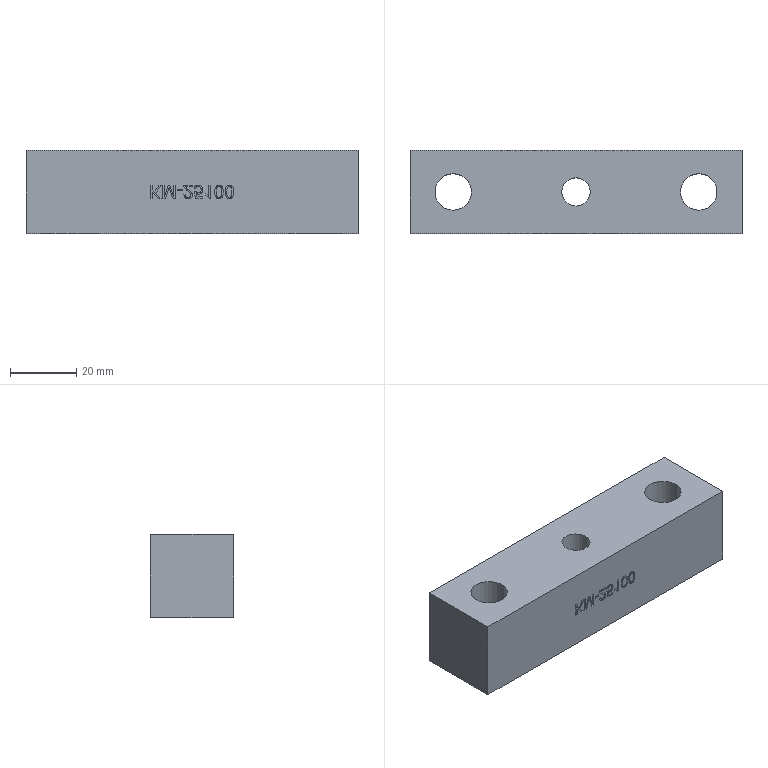Part | STEP file | lll_id1698_x_t | 1 solid | 86 faces | box 100 x 25 x 25 mm | volume 52659 mm3 | plane 62 | other 18 | cylinder 6 | commonest cylinder face diameters 11 x3 17 x2 8.5 x1